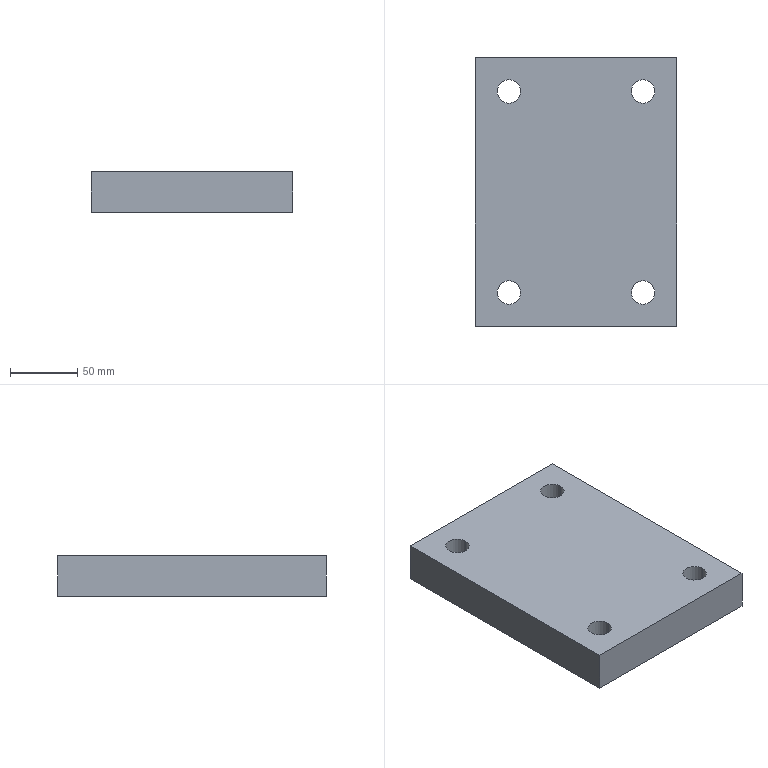Part | SolidWorks | features 3DProfileFeature 1, Extrusion 1, HoleWzd 1 | 1 solid | 14 faces | box 150 x 200 x 30 mm | volume 871137 mm3 | cylinder 8 | plane 6 | commonest cylinder face diameters 17.5 x8
STEP:
#1=CARTESIAN_POINT('',(16.25,175.,0.));
#2=VERTEX_POINT('',#1);
#3=CARTESIAN_POINT('',(33.75,175.,0.));
#4=VERTEX_POINT('',#3);
#5=CARTESIAN_POINT('',(25.,175.,0.));
#6=DIRECTION('',(0.,0.,1.));
#7=DIRECTION('',(1.,0.,0.));
#8=AXIS2_PLACEMENT_3D('',#5,#6,#7);
#9=CIRCLE('',#8,8.75);
#10=EDGE_CURVE('',#2,#4,#9,.T.);
#11=ORIENTED_EDGE('',*,*,#10,.F.);
#12=CARTESIAN_POINT('',(16.25,175.,30.));
#13=VERTEX_POINT('',#12);
#14=CARTESIAN_POINT('',(16.25,175.,30.));
#15=DIRECTION('',(0.,0.,1.));
#16=VECTOR('',#15,1000.);
#17=LINE('',#14,#16);
#18=EDGE_CURVE('',#2,#13,#17,.T.);
#19=ORIENTED_EDGE('',*,*,#18,.T.);
#20=CARTESIAN_POINT('',(33.75,175.,30.));
#21=VERTEX_POINT('',#20);
#22=CARTESIAN_POINT('',(25.,175.,30.));
#23=DIRECTION('',(0.,0.,1.));
#24=DIRECTION('',(1.,0.,0.));
#25=AXIS2_PLACEMENT_3D('',#22,#23,#24);
#26=CIRCLE('',#25,8.75);
#27=EDGE_CURVE('',#13,#21,#26,.T.);
#28=ORIENTED_EDGE('',*,*,#27,.T.);
#29=CARTESIAN_POINT('',(33.75,175.,30.));
#30=DIRECTION('',(0.,0.,1.));
#31=VECTOR('',#30,1000.);
#32=LINE('',#29,#31);
#33=EDGE_CURVE('',#4,#21,#32,.T.);
#34=ORIENTED_EDGE('',*,*,#33,.F.);
#35=EDGE_LOOP('',(#11,#19,#28,#34));
#36=FACE_OUTER_BOUND('',#35,.T.);
#37=CARTESIAN_POINT('',(25.,175.,30.));
#38=DIRECTION('',(0.,0.,1.));
#39=DIRECTION('',(1.,0.,0.));
#40=AXIS2_PLACEMENT_3D('',#37,#38,#39);
#41=CYLINDRICAL_SURFACE('',#40,8.75);
#42=ADVANCED_FACE('',(#36),#41,.F.);
#43=CARTESIAN_POINT('',(116.25,175.,0.));
#44=VERTEX_POINT('',#43);
#45=CARTESIAN_POINT('',(133.75,175.,0.));
#46=VERTEX_POINT('',#45);
#47=CARTESIAN_POINT('',(125.,175.,0.));
#48=DIRECTION('',(0.,0.,1.));
#49=DIRECTION('',(1.,0.,0.));
#50=AXIS2_PLACEMENT_3D('',#47,#48,#49);
#51=CIRCLE('',#50,8.75);
#52=EDGE_CURVE('',#44,#46,#51,.T.);
#53=ORIENTED_EDGE('',*,*,#52,.F.);
#54=CARTESIAN_POINT('',(116.25,175.,30.));
#55=VERTEX_POINT('',#54);
#56=CARTESIAN_POINT('',(116.25,175.,30.));
#57=DIRECTION('',(0.,0.,1.));
#58=VECTOR('',#57,1000.);
#59=LINE('',#56,#58);
#60=EDGE_CURVE('',#44,#55,#59,.T.);
#61=ORIENTED_EDGE('',*,*,#60,.T.);
#62=CARTESIAN_POINT('',(133.75,175.,30.));
#63=VERTEX_POINT('',#62);
#64=CARTESIAN_POINT('',(125.,175.,30.));
#65=DIRECTION('',(0.,0.,1.));
#66=DIRECTION('',(1.,0.,0.));
#67=AXIS2_PLACEMENT_3D('',#64,#65,#66);
#68=CIRCLE('',#67,8.75);
#69=EDGE_CURVE('',#55,#63,#68,.T.);
#70=ORIENTED_EDGE('',*,*,#69,.T.);
#71=CARTESIAN_POINT('',(133.75,175.,30.));
#72=DIRECTION('',(0.,0.,1.));
#73=VECTOR('',#72,1000.);
#74=LINE('',#71,#73);
#75=EDGE_CURVE('',#46,#63,#74,.T.);
#76=ORIENTED_EDGE('',*,*,#75,.F.);
#77=EDGE_LOOP('',(#53,#61,#70,#76));
#78=FACE_OUTER_BOUND('',#77,.T.);
#79=CARTESIAN_POINT('',(125.,175.,30.));
#80=DIRECTION('',(0.,0.,1.));
#81=DIRECTION('',(1.,0.,0.));
#82=AXIS2_PLACEMENT_3D('',#79,#80,#81);
#83=CYLINDRICAL_SURFACE('',#82,8.75);
#84=ADVANCED_FACE('',(#78),#83,.F.);
#85=CARTESIAN_POINT('',(16.25,25.,0.));
#86=VERTEX_POINT('',#85);
#87=CARTESIAN_POINT('',(33.75,25.,0.));
#88=VERTEX_POINT('',#87);
#89=CARTESIAN_POINT('',(25.,25.,0.));
#90=DIRECTION('',(0.,0.,1.));
#91=DIRECTION('',(1.,0.,0.));
#92=AXIS2_PLACEMENT_3D('',#89,#90,#91);
#93=CIRCLE('',#92,8.75);
#94=EDGE_CURVE('',#86,#88,#93,.T.);
#95=ORIENTED_EDGE('',*,*,#94,.F.);
#96=CARTESIAN_POINT('',(16.25,25.,30.));
#97=VERTEX_POINT('',#96);
#98=CARTESIAN_POINT('',(16.25,25.,30.));
#99=DIRECTION('',(0.,0.,1.));
#100=VECTOR('',#99,1000.);
#101=LINE('',#98,#100);
#102=EDGE_CURVE('',#86,#97,#101,.T.);
#103=ORIENTED_EDGE('',*,*,#102,.T.);
#104=CARTESIAN_POINT('',(33.75,25.,30.));
#105=VERTEX_POINT('',#104);
#106=CARTESIAN_POINT('',(25.,25.,30.));
#107=DIRECTION('',(0.,0.,1.));
#108=DIRECTION('',(1.,0.,0.));
#109=AXIS2_PLACEMENT_3D('',#106,#107,#108);
#110=CIRCLE('',#109,8.75);
#111=EDGE_CURVE('',#97,#105,#110,.T.);
#112=ORIENTED_EDGE('',*,*,#111,.T.);
#113=CARTESIAN_POINT('',(33.75,25.,30.));
#114=DIRECTION('',(0.,0.,1.));
#115=VECTOR('',#114,1000.);
#116=LINE('',#113,#115);
#117=EDGE_CURVE('',#88,#105,#116,.T.);
#118=ORIENTED_EDGE('',*,*,#117,.F.);
#119=EDGE_LOOP('',(#95,#103,#112,#118));
#120=FACE_OUTER_BOUND('',#119,.T.);
#121=CARTESIAN_POINT('',(25.,25.,30.));
#122=DIRECTION('',(0.,0.,1.));
#123=DIRECTION('',(1.,0.,0.));
#124=AXIS2_PLACEMENT_3D('',#121,#122,#123);
#125=CYLINDRICAL_SURFACE('',#124,8.75);
#126=ADVANCED_FACE('',(#120),#125,.F.);
#127=CARTESIAN_POINT('',(116.25,25.,0.));
#128=VERTEX_POINT('',#127);
#129=CARTESIAN_POINT('',(133.75,25.,0.));
#130=VERTEX_POINT('',#129);
#131=CARTESIAN_POINT('',(125.,25.,0.));
#132=DIRECTION('',(0.,0.,1.));
#133=DIRECTION('',(1.,0.,0.));
#134=AXIS2_PLACEMENT_3D('',#131,#132,#133);
#135=CIRCLE('',#134,8.75);
#136=EDGE_CURVE('',#128,#130,#135,.T.);
#137=ORIENTED_EDGE('',*,*,#136,.F.);
#138=CARTESIAN_POINT('',(116.25,25.,30.));
#139=VERTEX_POINT('',#138);
#140=CARTESIAN_POINT('',(116.25,25.,30.));
#141=DIRECTION('',(0.,0.,1.));
#142=VECTOR('',#141,1000.);
#143=LINE('',#140,#142);
#144=EDGE_CURVE('',#128,#139,#143,.T.);
#145=ORIENTED_EDGE('',*,*,#144,.T.);
#146=CARTESIAN_POINT('',(133.75,25.,30.));
#147=VERTEX_POINT('',#146);
#148=CARTESIAN_POINT('',(125.,25.,30.));
#149=DIRECTION('',(0.,0.,1.));
#150=DIRECTION('',(1.,0.,0.));
#151=AXIS2_PLACEMENT_3D('',#148,#149,#150);
#152=CIRCLE('',#151,8.75);
#153=EDGE_CURVE('',#139,#147,#152,.T.);
#154=ORIENTED_EDGE('',*,*,#153,.T.);
#155=CARTESIAN_POINT('',(133.75,25.,30.));
#156=DIRECTION('',(0.,0.,1.));
#157=VECTOR('',#156,1000.);
#158=LINE('',#155,#157);
#159=EDGE_CURVE('',#130,#147,#158,.T.);
#160=ORIENTED_EDGE('',*,*,#159,.F.);
#161=EDGE_LOOP('',(#137,#145,#154,#160));
#162=FACE_OUTER_BOUND('',#161,.T.);
#163=CARTESIAN_POINT('',(125.,25.,30.));
#164=DIRECTION('',(0.,0.,1.));
#165=DIRECTION('',(1.,0.,0.));
#166=AXIS2_PLACEMENT_3D('',#163,#164,#165);
#167=CYLINDRICAL_SURFACE('',#166,8.75);
#168=ADVANCED_FACE('',(#162),#167,.F.);
#169=CARTESIAN_POINT('',(0.,200.,0.));
#170=VERTEX_POINT('',#169);
#171=CARTESIAN_POINT('',(0.,0.,0.));
#172=VERTEX_POINT('',#171);
#173=CARTESIAN_POINT('',(0.,0.,0.));
#174=DIRECTION('',(0.,-1.,0.));
#175=VECTOR('',#174,1000.);
#176=LINE('',#173,#175);
#177=EDGE_CURVE('',#170,#172,#176,.T.);
#178=ORIENTED_EDGE('',*,*,#177,.T.);
#179=CARTESIAN_POINT('',(0.,0.,30.));
#180=VERTEX_POINT('',#179);
#181=CARTESIAN_POINT('',(0.,0.,30.));
#182=DIRECTION('',(0.,0.,-1.));
#183=VECTOR('',#182,1000.);
#184=LINE('',#181,#183);
#185=EDGE_CURVE('',#180,#172,#184,.T.);
#186=ORIENTED_EDGE('',*,*,#185,.F.);
#187=CARTESIAN_POINT('',(0.,200.,30.));
#188=VERTEX_POINT('',#187);
#189=CARTESIAN_POINT('',(0.,0.,30.));
#190=DIRECTION('',(0.,-1.,0.));
#191=VECTOR('',#190,1000.);
#192=LINE('',#189,#191);
#193=EDGE_CURVE('',#188,#180,#192,.T.);
#194=ORIENTED_EDGE('',*,*,#193,.F.);
#195=CARTESIAN_POINT('',(0.,200.,30.));
#196=DIRECTION('',(0.,0.,-1.));
#197=VECTOR('',#196,1000.);
#198=LINE('',#195,#197);
#199=EDGE_CURVE('',#188,#170,#198,.T.);
#200=ORIENTED_EDGE('',*,*,#199,.T.);
#201=EDGE_LOOP('',(#178,#186,#194,#200));
#202=FACE_OUTER_BOUND('',#201,.T.);
#203=CARTESIAN_POINT('',(0.,0.,30.));
#204=DIRECTION('',(1.,0.,0.));
#205=DIRECTION('',(0.,0.,-1.));
#206=AXIS2_PLACEMENT_3D('',#203,#204,#205);
#207=PLANE('',#206);
#208=ADVANCED_FACE('',(#202),#207,.F.);
#209=CARTESIAN_POINT('',(150.,0.,0.));
#210=VERTEX_POINT('',#209);
#211=CARTESIAN_POINT('',(0.,0.,0.));
#212=DIRECTION('',(1.,0.,0.));
#213=VECTOR('',#212,1000.);
#214=LINE('',#211,#213);
#215=EDGE_CURVE('',#172,#210,#214,.T.);
#216=ORIENTED_EDGE('',*,*,#215,.T.);
#217=CARTESIAN_POINT('',(150.,0.,30.));
#218=VERTEX_POINT('',#217);
#219=CARTESIAN_POINT('',(150.,0.,30.));
#220=DIRECTION('',(0.,0.,-1.));
#221=VECTOR('',#220,1000.);
#222=LINE('',#219,#221);
#223=EDGE_CURVE('',#218,#210,#222,.T.);
#224=ORIENTED_EDGE('',*,*,#223,.F.);
#225=CARTESIAN_POINT('',(0.,0.,30.));
#226=DIRECTION('',(1.,0.,0.));
#227=VECTOR('',#226,1000.);
#228=LINE('',#225,#227);
#229=EDGE_CURVE('',#180,#218,#228,.T.);
#230=ORIENTED_EDGE('',*,*,#229,.F.);
#231=ORIENTED_EDGE('',*,*,#185,.T.);
#232=EDGE_LOOP('',(#216,#224,#230,#231));
#233=FACE_OUTER_BOUND('',#232,.T.);
#234=CARTESIAN_POINT('',(0.,0.,30.));
#235=DIRECTION('',(0.,1.,0.));
#236=DIRECTION('',(0.,0.,1.));
#237=AXIS2_PLACEMENT_3D('',#234,#235,#236);
#238=PLANE('',#237);
#239=ADVANCED_FACE('',(#233),#238,.F.);
#240=CARTESIAN_POINT('',(150.,200.,0.));
#241=VERTEX_POINT('',#240);
#242=CARTESIAN_POINT('',(150.,0.,0.));
#243=DIRECTION('',(0.,1.,0.));
#244=VECTOR('',#243,1000.);
#245=LINE('',#242,#244);
#246=EDGE_CURVE('',#210,#241,#245,.T.);
#247=ORIENTED_EDGE('',*,*,#246,.T.);
#248=CARTESIAN_POINT('',(150.,200.,30.));
#249=VERTEX_POINT('',#248);
#250=CARTESIAN_POINT('',(150.,200.,30.));
#251=DIRECTION('',(0.,0.,-1.));
#252=VECTOR('',#251,1000.);
#253=LINE('',#250,#252);
#254=EDGE_CURVE('',#249,#241,#253,.T.);
#255=ORIENTED_EDGE('',*,*,#254,.F.);
#256=CARTESIAN_POINT('',(150.,0.,30.));
#257=DIRECTION('',(0.,1.,0.));
#258=VECTOR('',#257,1000.);
#259=LINE('',#256,#258);
#260=EDGE_CURVE('',#218,#249,#259,.T.);
#261=ORIENTED_EDGE('',*,*,#260,.F.);
#262=ORIENTED_EDGE('',*,*,#223,.T.);
#263=EDGE_LOOP('',(#247,#255,#261,#262));
#264=FACE_OUTER_BOUND('',#263,.T.);
#265=CARTESIAN_POINT('',(150.,0.,30.));
#266=DIRECTION('',(-1.,0.,0.));
#267=DIRECTION('',(0.,0.,1.));
#268=AXIS2_PLACEMENT_3D('',#265,#266,#267);
#269=PLANE('',#268);
#270=ADVANCED_FACE('',(#264),#269,.F.);
#271=CARTESIAN_POINT('',(0.,200.,0.));
#272=DIRECTION('',(-1.,0.,0.));
#273=VECTOR('',#272,1000.);
#274=LINE('',#271,#273);
#275=EDGE_CURVE('',#241,#170,#274,.T.);
#276=ORIENTED_EDGE('',*,*,#275,.T.);
#277=ORIENTED_EDGE('',*,*,#199,.F.);
#278=CARTESIAN_POINT('',(0.,200.,30.));
#279=DIRECTION('',(-1.,0.,0.));
#280=VECTOR('',#279,1000.);
#281=LINE('',#278,#280);
#282=EDGE_CURVE('',#249,#188,#281,.T.);
#283=ORIENTED_EDGE('',*,*,#282,.F.);
#284=ORIENTED_EDGE('',*,*,#254,.T.);
#285=EDGE_LOOP('',(#276,#277,#283,#284));
#286=FACE_OUTER_BOUND('',#285,.T.);
#287=CARTESIAN_POINT('',(0.,200.,30.));
#288=DIRECTION('',(0.,-1.,0.));
#289=DIRECTION('',(0.,0.,-1.));
#290=AXIS2_PLACEMENT_3D('',#287,#288,#289);
#291=PLANE('',#290);
#292=ADVANCED_FACE('',(#286),#291,.F.);
#293=CARTESIAN_POINT('',(25.,175.,30.));
#294=DIRECTION('',(0.,0.,1.));
#295=DIRECTION('',(1.,0.,0.));
#296=AXIS2_PLACEMENT_3D('',#293,#294,#295);
#297=CIRCLE('',#296,8.75);
#298=EDGE_CURVE('',#21,#13,#297,.T.);
#299=ORIENTED_EDGE('',*,*,#298,.F.);
#300=ORIENTED_EDGE('',*,*,#27,.F.);
#301=EDGE_LOOP('',(#299,#300));
#302=FACE_BOUND('',#301,.T.);
#303=CARTESIAN_POINT('',(125.,175.,30.));
#304=DIRECTION('',(0.,0.,1.));
#305=DIRECTION('',(1.,0.,0.));
#306=AXIS2_PLACEMENT_3D('',#303,#304,#305);
#307=CIRCLE('',#306,8.75);
#308=EDGE_CURVE('',#63,#55,#307,.T.);
#309=ORIENTED_EDGE('',*,*,#308,.F.);
#310=ORIENTED_EDGE('',*,*,#69,.F.);
#311=EDGE_LOOP('',(#309,#310));
#312=FACE_BOUND('',#311,.T.);
#313=CARTESIAN_POINT('',(25.,25.,30.));
#314=DIRECTION('',(0.,0.,1.));
#315=DIRECTION('',(1.,0.,0.));
#316=AXIS2_PLACEMENT_3D('',#313,#314,#315);
#317=CIRCLE('',#316,8.75);
#318=EDGE_CURVE('',#105,#97,#317,.T.);
#319=ORIENTED_EDGE('',*,*,#318,.F.);
#320=ORIENTED_EDGE('',*,*,#111,.F.);
#321=EDGE_LOOP('',(#319,#320));
#322=FACE_BOUND('',#321,.T.);
#323=CARTESIAN_POINT('',(125.,25.,30.));
#324=DIRECTION('',(0.,0.,1.));
#325=DIRECTION('',(1.,0.,0.));
#326=AXIS2_PLACEMENT_3D('',#323,#324,#325);
#327=CIRCLE('',#326,8.75);
#328=EDGE_CURVE('',#147,#139,#327,.T.);
#329=ORIENTED_EDGE('',*,*,#328,.F.);
#330=ORIENTED_EDGE('',*,*,#153,.F.);
#331=EDGE_LOOP('',(#329,#330));
#332=FACE_BOUND('',#331,.T.);
#333=ORIENTED_EDGE('',*,*,#193,.T.);
#334=ORIENTED_EDGE('',*,*,#229,.T.);
#335=ORIENTED_EDGE('',*,*,#260,.T.);
#336=ORIENTED_EDGE('',*,*,#282,.T.);
#337=EDGE_LOOP('',(#333,#334,#335,#336));
#338=FACE_OUTER_BOUND('',#337,.T.);
#339=CARTESIAN_POINT('',(0.,0.,30.));
#340=DIRECTION('',(0.,0.,-1.));
#341=DIRECTION('',(-1.,0.,0.));
#342=AXIS2_PLACEMENT_3D('',#339,#340,#341);
#343=PLANE('',#342);
#344=ADVANCED_FACE('',(#302,#312,#322,#332,#338),#343,.F.);
#345=CARTESIAN_POINT('',(25.,175.,0.));
#346=DIRECTION('',(0.,0.,1.));
#347=DIRECTION('',(1.,0.,0.));
#348=AXIS2_PLACEMENT_3D('',#345,#346,#347);
#349=CIRCLE('',#348,8.75);
#350=EDGE_CURVE('',#4,#2,#349,.T.);
#351=ORIENTED_EDGE('',*,*,#350,.T.);
#352=ORIENTED_EDGE('',*,*,#10,.T.);
#353=EDGE_LOOP('',(#351,#352));
#354=FACE_BOUND('',#353,.T.);
#355=CARTESIAN_POINT('',(125.,175.,0.));
#356=DIRECTION('',(0.,0.,1.));
#357=DIRECTION('',(1.,0.,0.));
#358=AXIS2_PLACEMENT_3D('',#355,#356,#357);
#359=CIRCLE('',#358,8.75);
#360=EDGE_CURVE('',#46,#44,#359,.T.);
#361=ORIENTED_EDGE('',*,*,#360,.T.);
#362=ORIENTED_EDGE('',*,*,#52,.T.);
#363=EDGE_LOOP('',(#361,#362));
#364=FACE_BOUND('',#363,.T.);
#365=CARTESIAN_POINT('',(25.,25.,0.));
#366=DIRECTION('',(0.,0.,1.));
#367=DIRECTION('',(1.,0.,0.));
#368=AXIS2_PLACEMENT_3D('',#365,#366,#367);
#369=CIRCLE('',#368,8.75);
#370=EDGE_CURVE('',#88,#86,#369,.T.);
#371=ORIENTED_EDGE('',*,*,#370,.T.);
#372=ORIENTED_EDGE('',*,*,#94,.T.);
#373=EDGE_LOOP('',(#371,#372));
#374=FACE_BOUND('',#373,.T.);
#375=CARTESIAN_POINT('',(125.,25.,0.));
#376=DIRECTION('',(0.,0.,1.));
#377=DIRECTION('',(1.,0.,0.));
#378=AXIS2_PLACEMENT_3D('',#375,#376,#377);
#379=CIRCLE('',#378,8.75);
#380=EDGE_CURVE('',#130,#128,#379,.T.);
#381=ORIENTED_EDGE('',*,*,#380,.T.);
#382=ORIENTED_EDGE('',*,*,#136,.T.);
#383=EDGE_LOOP('',(#381,#382));
#384=FACE_BOUND('',#383,.T.);
#385=ORIENTED_EDGE('',*,*,#177,.F.);
#386=ORIENTED_EDGE('',*,*,#275,.F.);
#387=ORIENTED_EDGE('',*,*,#246,.F.);
#388=ORIENTED_EDGE('',*,*,#215,.F.);
#389=EDGE_LOOP('',(#385,#386,#387,#388));
#390=FACE_OUTER_BOUND('',#389,.T.);
#391=CARTESIAN_POINT('',(0.,0.,0.));
#392=DIRECTION('',(0.,0.,-1.));
#393=DIRECTION('',(-1.,0.,0.));
#394=AXIS2_PLACEMENT_3D('',#391,#392,#393);
#395=PLANE('',#394);
#396=ADVANCED_FACE('',(#354,#364,#374,#384,#390),#395,.T.);
#397=ORIENTED_EDGE('',*,*,#144,.F.);
#398=ORIENTED_EDGE('',*,*,#380,.F.);
#399=ORIENTED_EDGE('',*,*,#159,.T.);
#400=ORIENTED_EDGE('',*,*,#328,.T.);
#401=EDGE_LOOP('',(#397,#398,#399,#400));
#402=FACE_OUTER_BOUND('',#401,.T.);
#403=CARTESIAN_POINT('',(125.,25.,30.));
#404=DIRECTION('',(0.,0.,1.));
#405=DIRECTION('',(1.,0.,0.));
#406=AXIS2_PLACEMENT_3D('',#403,#404,#405);
#407=CYLINDRICAL_SURFACE('',#406,8.75);
#408=ADVANCED_FACE('',(#402),#407,.F.);
#409=ORIENTED_EDGE('',*,*,#102,.F.);
#410=ORIENTED_EDGE('',*,*,#370,.F.);
#411=ORIENTED_EDGE('',*,*,#117,.T.);
#412=ORIENTED_EDGE('',*,*,#318,.T.);
#413=EDGE_LOOP('',(#409,#410,#411,#412));
#414=FACE_OUTER_BOUND('',#413,.T.);
#415=CARTESIAN_POINT('',(25.,25.,30.));
#416=DIRECTION('',(0.,0.,1.));
#417=DIRECTION('',(1.,0.,0.));
#418=AXIS2_PLACEMENT_3D('',#415,#416,#417);
#419=CYLINDRICAL_SURFACE('',#418,8.75);
#420=ADVANCED_FACE('',(#414),#419,.F.);
#421=ORIENTED_EDGE('',*,*,#60,.F.);
#422=ORIENTED_EDGE('',*,*,#360,.F.);
#423=ORIENTED_EDGE('',*,*,#75,.T.);
#424=ORIENTED_EDGE('',*,*,#308,.T.);
#425=EDGE_LOOP('',(#421,#422,#423,#424));
#426=FACE_OUTER_BOUND('',#425,.T.);
#427=CARTESIAN_POINT('',(125.,175.,30.));
#428=DIRECTION('',(0.,0.,1.));
#429=DIRECTION('',(1.,0.,0.));
#430=AXIS2_PLACEMENT_3D('',#427,#428,#429);
#431=CYLINDRICAL_SURFACE('',#430,8.75);
#432=ADVANCED_FACE('',(#426),#431,.F.);
#433=ORIENTED_EDGE('',*,*,#18,.F.);
#434=ORIENTED_EDGE('',*,*,#350,.F.);
#435=ORIENTED_EDGE('',*,*,#33,.T.);
#436=ORIENTED_EDGE('',*,*,#298,.T.);
#437=EDGE_LOOP('',(#433,#434,#435,#436));
#438=FACE_OUTER_BOUND('',#437,.T.);
#439=CARTESIAN_POINT('',(25.,175.,30.));
#440=DIRECTION('',(0.,0.,1.));
#441=DIRECTION('',(1.,0.,0.));
#442=AXIS2_PLACEMENT_3D('',#439,#440,#441);
#443=CYLINDRICAL_SURFACE('',#442,8.75);
#444=ADVANCED_FACE('',(#438),#443,.F.);
#445=CLOSED_SHELL('',(#42,#84,#126,#168,#208,#239,#270,#292,#344,#396,#408,#420,#432,#444));
#446=MANIFOLD_SOLID_BREP('',#445);
#447=CARTESIAN_POINT('',(0.,0.,0.));
#448=DIRECTION('',(0.,0.,1.));
#449=DIRECTION('',(1.,0.,0.));
#450=AXIS2_PLACEMENT_3D('',#447,#448,#449);
#451=(LENGTH_UNIT()NAMED_UNIT(*)SI_UNIT(.MILLI.,.METRE.));
#452=UNCERTAINTY_MEASURE_WITH_UNIT(LENGTH_MEASURE(0.00001),#451,'','');
#453=(NAMED_UNIT(*)PLANE_ANGLE_UNIT()SI_UNIT($,.RADIAN.));
#454=(NAMED_UNIT(*)SI_UNIT($,.STERADIAN.)SOLID_ANGLE_UNIT());
#455=(GEOMETRIC_REPRESENTATION_CONTEXT(3)GLOBAL_UNCERTAINTY_ASSIGNED_CONTEXT((#452))GLOBAL_UNIT_ASSIGNED_CONTEXT((#451,#453,#454))REPRESENTATION_CONTEXT('',''));
#456=ADVANCED_BREP_SHAPE_REPRESENTATION('',(#446,#450),#455);